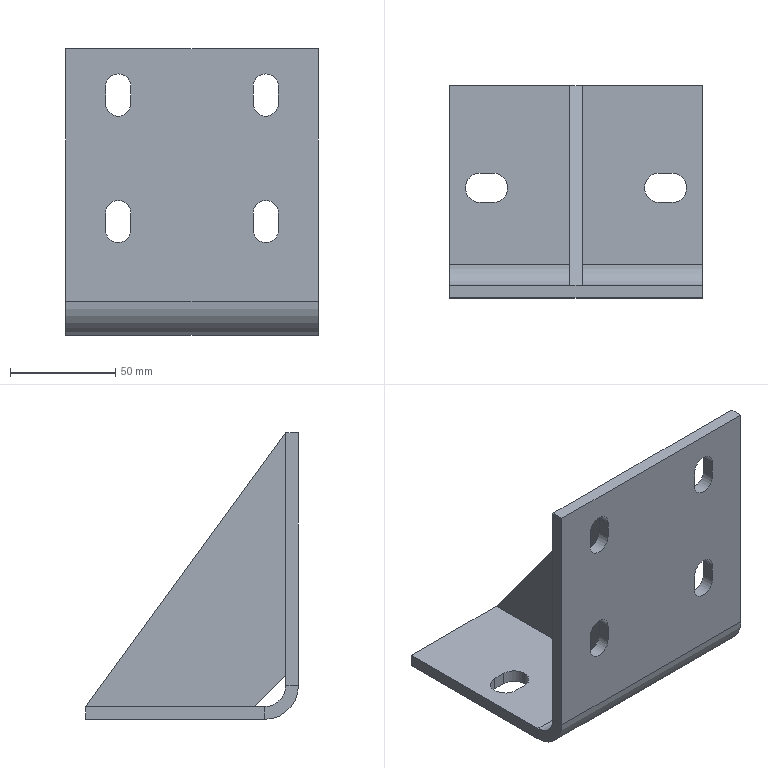Part | STEP file | Guide shoe lower bracket | 1 solid | 48 faces | box 120 x 101 x 136 mm | volume 190804 mm3 | plane 28 | cylinder 20 | commonest cylinder face diameters 12 x12 14 x6 20 x1 32 x1